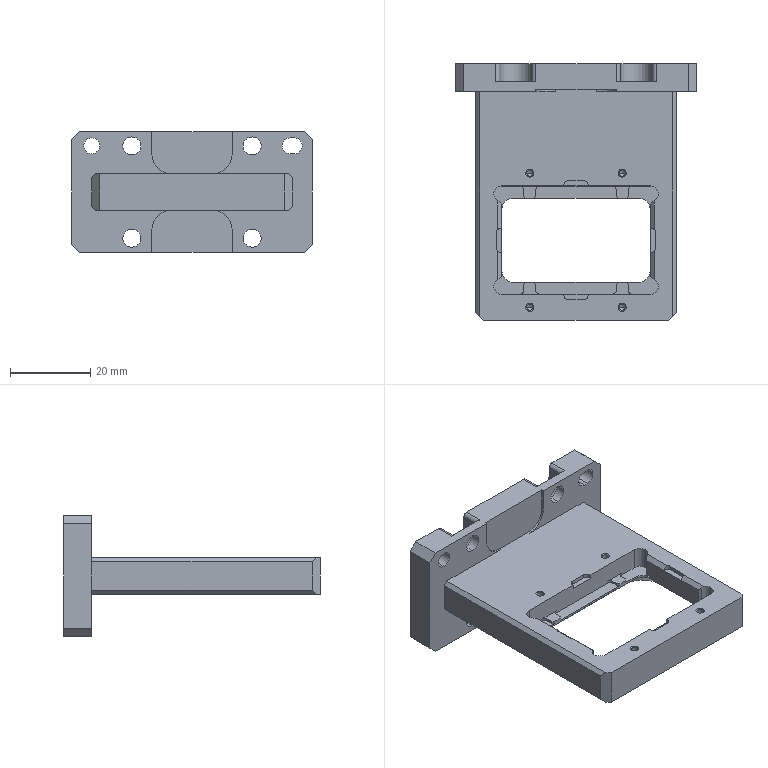Part | 1 solid | 186 faces | box 60 x 64 x 30 mm | volume 27587 mm3 | plane 102 | cylinder 64 | cone 20 | commonest cylinder face diameters 2 x24 4 x10 1.6 x8 4.5 x8 8 x6 6 x4